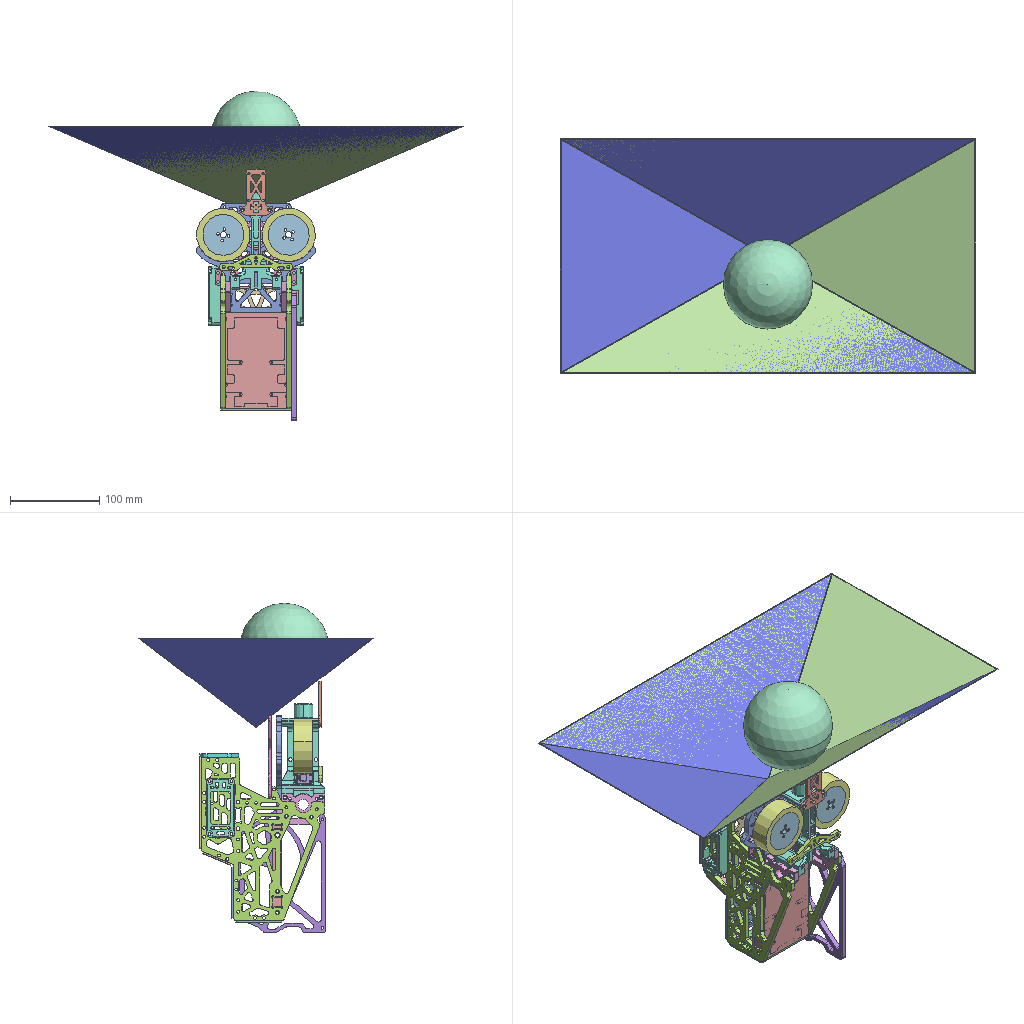Assembly | SolidWorks | 37 different items | 43 placed | box 466 x 263 x 369 mm
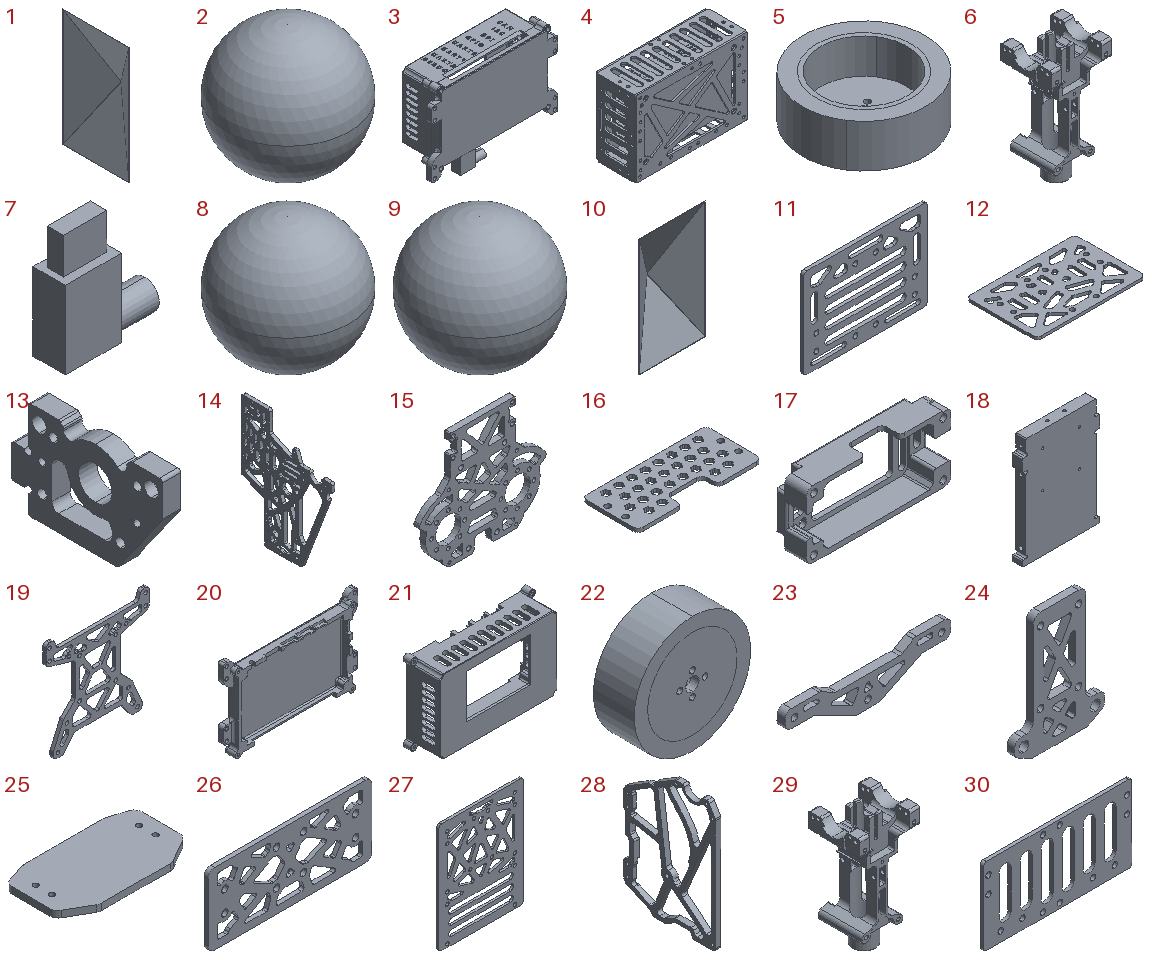Parts list (item | name | quantity | parent item | size | volume | features):
1 | (subassembly) | x1 | - | 100 x 263.013 x 465.513 mm | 119004 mm3 | -
2 | (subassembly) | x1 | - | 100 x 100 x 100 mm | 589049 mm3 | -
3 | (subassembly) | x1 | - | 126 x 39.5 x 91.6 mm | 67574 mm3 | -
4 | (subassembly) | x1 | - | 136 x 50 x 97 mm | 125770 mm3 | -
5 | (subassembly) | x2 | - | 60 x 60 x 21 mm | 35557 mm3 | -
6 | (subassembly) | x1 | - | 60 x 48 x 108.75 mm | 36754 mm3 | -
7 | - | x1 | - | 26.5 x 9 x 31.5 mm | 4092 mm3 | features ICE 2, Extrusion 1
8 | - | x1 | in 2 | 100 x 100 x 100 mm | 523599 mm3 | features Revolution 1
9 | - | x1 | in 2 | 50 x 50 x 50 mm | 65450 mm3 | features Revolution 1
10 | - | x1 | in 1 | 263.013 x 100 x 465.513 mm | 119004 mm3 | features 3DProfileFeature 5, CirPattern 2, FillRefSurface 2, Thicken 2, RefAxis 1
11 | - | x1 | - | 79 x 2 x 57.5 mm | 5646 mm3 | features Extrusion 1, Fillet 1, ICE 1
12 | - | x1 | - | 79 x 51.5 x 2 mm | 5613 mm3 | features Fillet 5, ICE 3, Extrusion 1
13 | - | x2 | - | 6.5 x 54 x 35 mm | 7066 mm3 | features HoleWzd 3, Fillet 2, Chamfer 1, Extrusion 1
14 | - | x2 | - | 5 x 138 x 183 mm | 44741 mm3 | features Fillet 3, Extrusion 1, ICE 1
15 | - | x1 | - | 133.928 x 6 x 121.75 mm | 39124 mm3 | features Fillet 3, ICE 2, Extrusion 1
16 | - | x1 | - | 69 x 31.5 x 2 mm | 3100 mm3 | features Fillet 2, Extrusion 1, ICE 1
17 | - | x2 | - | 66 x 14 x 30.5 mm | 6792 mm3 | features ICE 14, Fillet 6, Chamfer 1, Extrusion 1
18 | - | x1 | - | 76 x 10 x 107.5 mm | 24777 mm3 | features HoleWzd 5, Fillet 2, Extrusion 1, ICE 1
19 | - | x1 | - | 91 x 3 x 91.75 mm | 7865 mm3 | features Fillet 2, Extrusion 1, ICE 1
20 | - | x1 | - | 126 x 9.5 x 78.6 mm | 28044 mm3 | features Fillet 7, ICE 4, Cut 2, MBimport 1, MirrorPattern 1
21 | - | x1 | - | 113.2 x 30 x 73.2 mm | 35438 mm3 | features BaseBody 1, Chamfer 1, ICE 1
22 | - | x2 | in 5 | 60 x 21 x 60 mm | 35557 mm3 | features ICE 2, Extrusion 1
23 | - | x1 | - | 81 x 4 x 18.75 mm | 2669 mm3 | features Fillet 2, Extrusion 1, ICE 1
24 | - | x1 | - | 38 x 3 x 51.4 mm | 2836 mm3 | features Fillet 2, Extrusion 1, ICE 1
25 | - | x1 | - | 79 x 44 x 4 mm | 12779 mm3 | features Extrusion 1, Fillet 1
26 | - | x1 | - | 79 x 2 x 34.5 mm | 3709 mm3 | features Fillet 2, Extrusion 1, ICE 1
27 | - | x1 | - | 79 x 2 x 102.5 mm | 10788 mm3 | features Fillet 2, Extrusion 1, ICE 1
28 | - | x1 | - | 6 x 103 x 144 mm | 23755 mm3 | features Fillet 3, ICE 2, Extrusion 1, HoleWzd 1
29 | - | x1 | in 6 | 60 x 48 x 108.75 mm | 35872 mm3 | features ICE 19, Fillet 6, HoleWzd 4, MirrorPattern 4, Chamfer 3, 3DProfileFeature 1, Extrusion 1
30 | - | x1 | - | 88.5 x 2 x 46 mm | 5464 mm3 | features Extrusion 1, Fillet 1, ICE 1
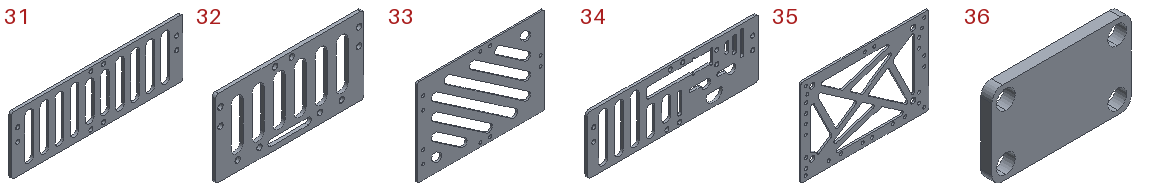31 | - | x1 | - | 136 x 2 x 46 mm | 7575 mm3 | features Extrusion 1, Fillet 1, ICE 1
32 | - | x1 | - | 88.5 x 2 x 46 mm | 5379 mm3 | features Extrusion 1, Fillet 1, ICE 1
33 | - | x1 | - | 134 x 2 x 91.5 mm | 16934 mm3 | features Fillet 4, ICE 2, Extrusion 1
34 | - | x1 | - | 136 x 2 x 46 mm | 8461 mm3 | features Fillet 2, Extrusion 1, ICE 1
35 | - | x1 | - | 136 x 2 x 92.5 mm | 14381 mm3 | features Fillet 2, Extrusion 1, ICE 1
36 | - | x2 | in 6 | 20 x 5.45 x 12 mm | 441.181 mm3 | features ICE 3, Fillet 2, Extrusion 1, Revolution 1
37 | Mini PC NX Assembly Unit (subassembly) | x1 | - | - | - | -
Mates (type | each side: item.copy, entity, surface, feature):
In the top assembly
Parallel | 18.1 face plane Boss-Extrude1 | assembly plane | 2 times
Coincident | 18.1 face plane Boss-Extrude1 | 14.1 face plane Boss-Extrude1
Concentric | assembly face | 15.1 face cylinder Boss-Extrude1 | 4 times
Coincident | assembly face | 15.1 face plane Boss-Extrude1 | 2 times
Concentric | assembly face | 19.1 face cylinder Boss-Extrude1 | 2 times
Coincident | assembly face | 19.1 face plane Boss-Extrude1
Coincident | 18.1 face plane Boss-Extrude1 | 14.2 face plane Boss-Extrude1
Concentric | 18.1 face cylinder M5 Tapped Hole1 | 14.2 face cylinder Boss-Extrude1
Concentric | 18.1 face cylinder M5 Tapped Hole1 | 14.1 face cylinder Boss-Extrude1
Coincident | 14.2 face plane Boss-Extrude1 | 13.1 face plane Boss-Extrude1
Concentric | 18.1 face cylinder M4 Tapped Hole2 | 14.1 face cylinder Boss-Extrude1
Concentric | 18.1 face cylinder M4 Tapped Hole1 | 14.2 face cylinder Boss-Extrude1
Concentric | 14.2 face cylinder Boss-Extrude1 | 13.1 face cylinder M3 Tapped Hole1
Concentric | 18.1 face cylinder M3 Tapped Hole1 | 12.1 face cylinder Boss-Extrude1 | 2 times
Coincident | 18.1 face plane Boss-Extrude1 | 12.1 face plane Boss-Extrude1
Coincident | 14.2 face plane Boss-Extrude1 | 28.1 face plane Boss-Extrude1
Concentric | 14.2 face cylinder Boss-Extrude1 | 28.1 face cylinder Boss-Extrude1 | 2 times
Concentric | assembly face | 28.1 face cylinder Boss-Extrude1 | 2 times
Coincident | assembly face | 28.1 face plane Boss-Extrude1
Coincident | 6.1 select_type:25 | assembly select_type:11
Parallel | 29.1 face plane Main body | assembly plane | 2 times
Coincident | 29.1 face plane Main body | assembly face
Concentric | 29.1 face cylinder Barrel | assembly face
Coincident | assembly face | 24.1 face plane Boss-Extrude1
Concentric | 29.1 face cylinder Upper M4 threaded hole | 24.1 face cylinder Boss-Extrude1 | 2 times
Concentric | 13.1 face cylinder Boss-Extrude1 | 29.1 face cylinder Side M4 threaded hole | 2 times
Coincident | 13.1 face plane Boss-Extrude1 | 29.1 face plane Main body
Coincident | 15.1 face plane Boss-Extrude1 | 29.1 face plane Main body
Concentric | 15.1 face cylinder Boss-Extrude1 | 29.1 face cylinder Upper M4 threaded hole | 2 times
Coincident | 14.1 face plane Boss-Extrude1 | 13.2 face plane Boss-Extrude1
Concentric | 13.2 face cylinder Boss-Extrude1 | 29.1 face cylinder Side M4 threaded hole
Coincident | 29.1 face plane Upper/lower cut-through | 23.1 face plane Boss-Extrude1
Concentric | 15.1 face cylinder Boss-Extrude1 | 23.1 face cylinder Boss-Extrude1 | 2 times
Coincident | 14.2 face plane Boss-Extrude1 | 17.1 face plane Boss-Extrude1
Concentric | 14.2 face cylinder Boss-Extrude1 | 17.1 face cylinder Boss-Extrude1 | 2 times
Coincident | 14.1 face plane Boss-Extrude1 | 17.2 face plane Boss-Extrude1
Concentric | 14.1 face cylinder Boss-Extrude1 | 17.2 face cylinder Boss-Extrude1 | 2 times
In subassembly 6
Coincident | 29.2 select_type:25 | 6.2 select_type:11
Parallel | 29.2 face plane Main body | 6.2 plane
Concentric | 29.2 face cylinder Fluorescent charging M2.5 threaded hole | 36.1 face cylinder Screw hole | 2 times
Coincident | 29.2 face plane One-side fluorescent charging aluminium board cutout | 36.1 face plane Aluminium base plate
Concentric | 29.2 face cylinder Fluorescent charging M2.5 threaded hole | 36.2 face cylinder Screw hole | 2 times
Coincident | 29.2 face plane Opposite-side fluorescent charging aluminium board cutout | 36.2 face plane Aluminium base plate
In subassembly 2
Coordinate | 9.1 select_type:25 | 8.1 select_type:25